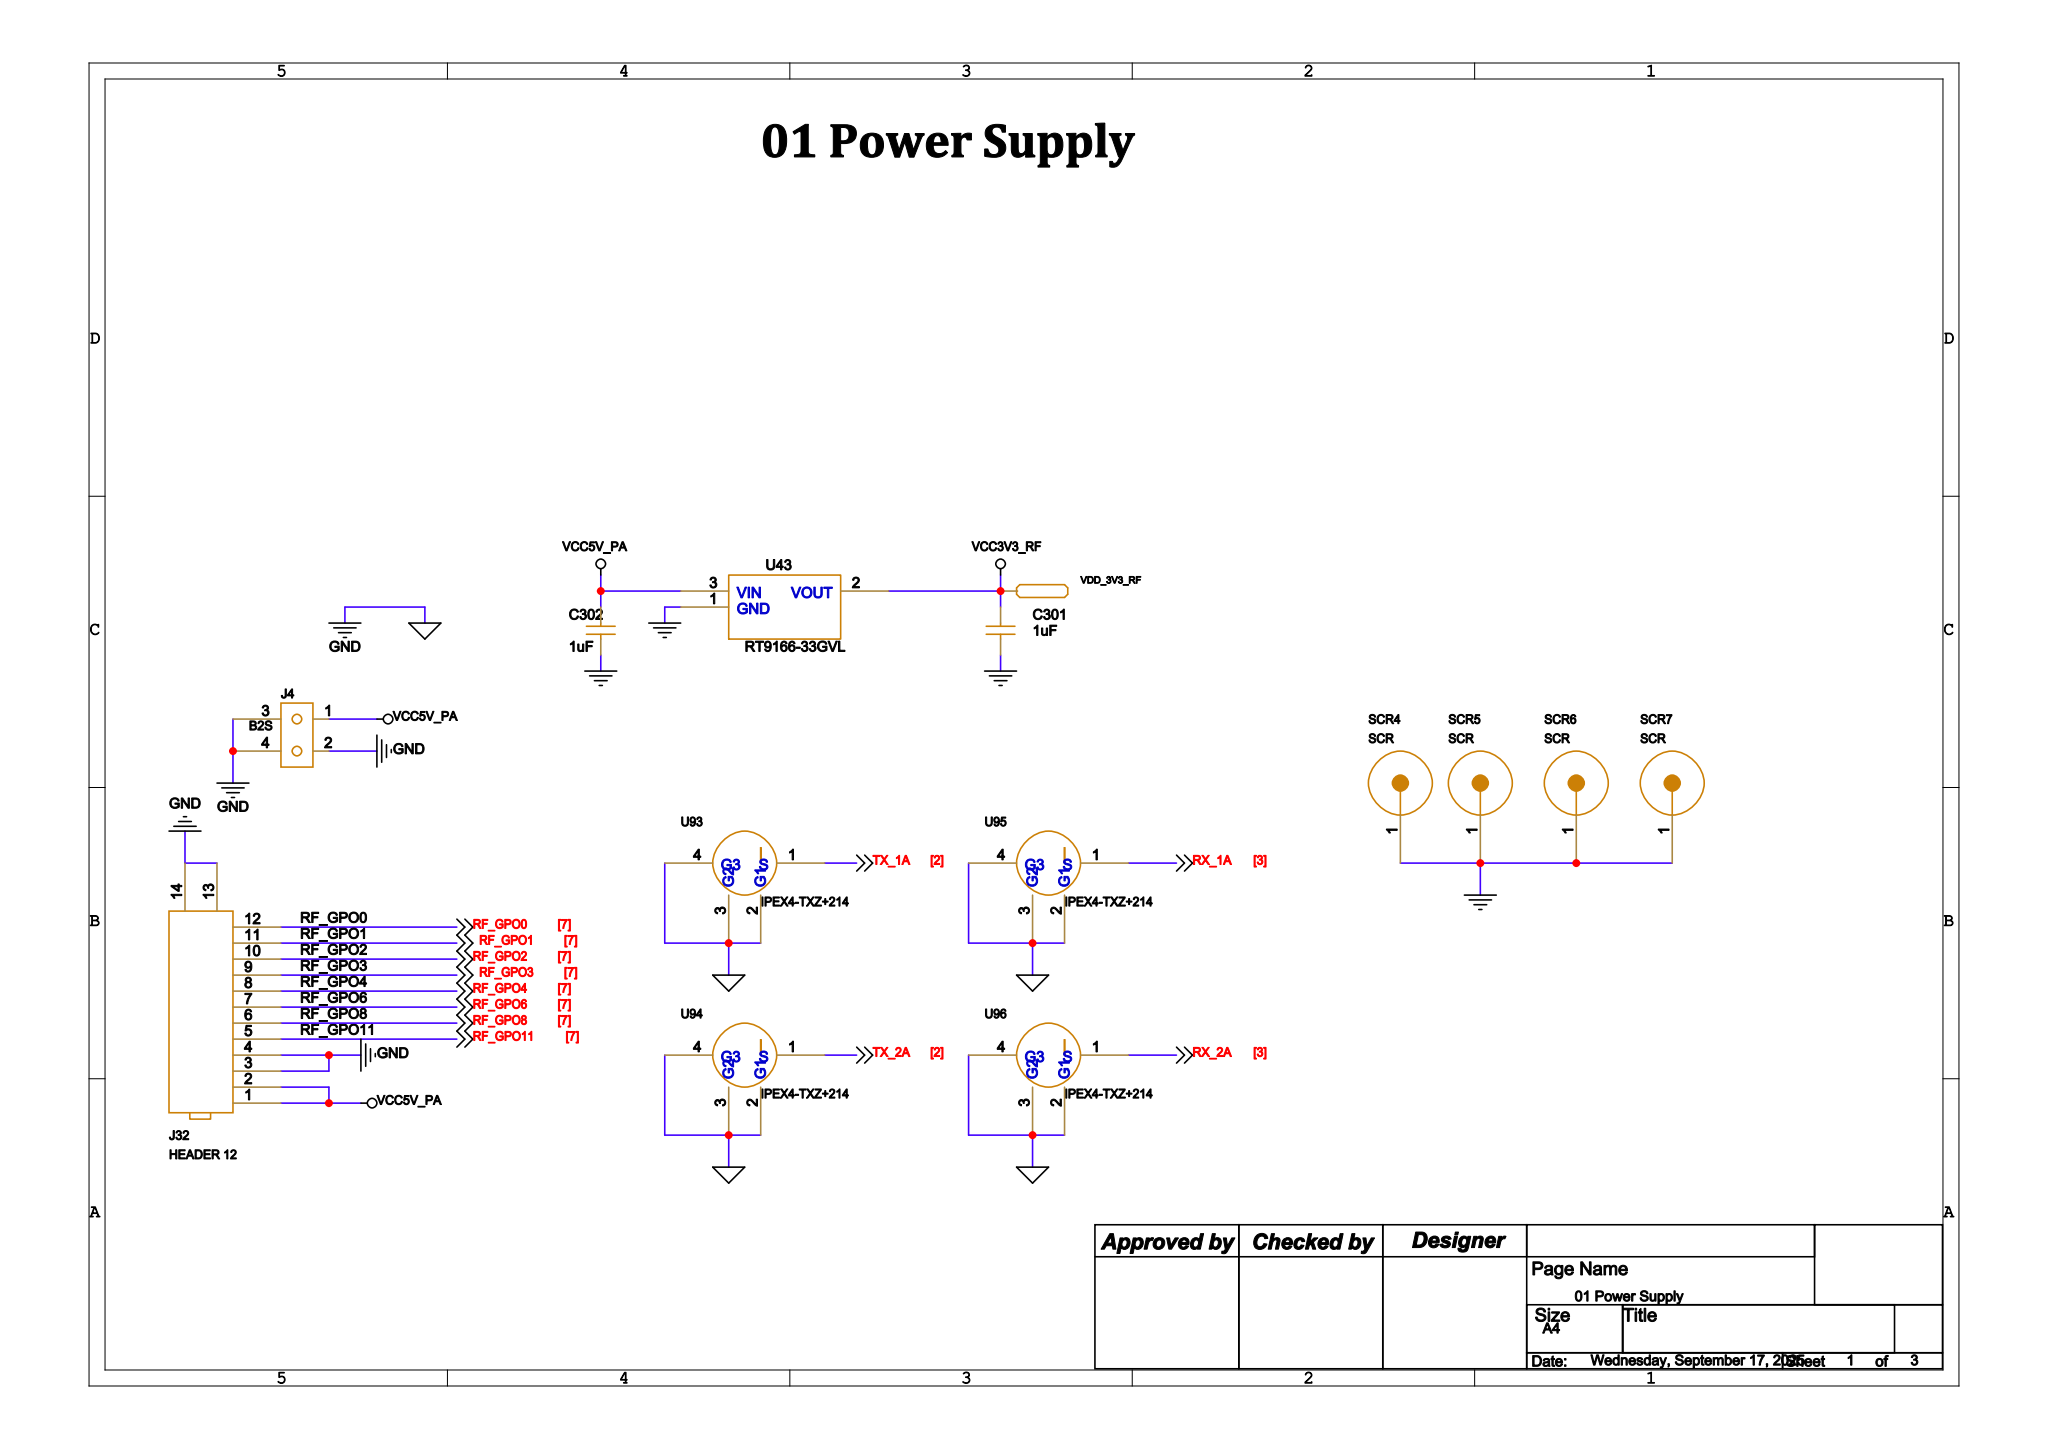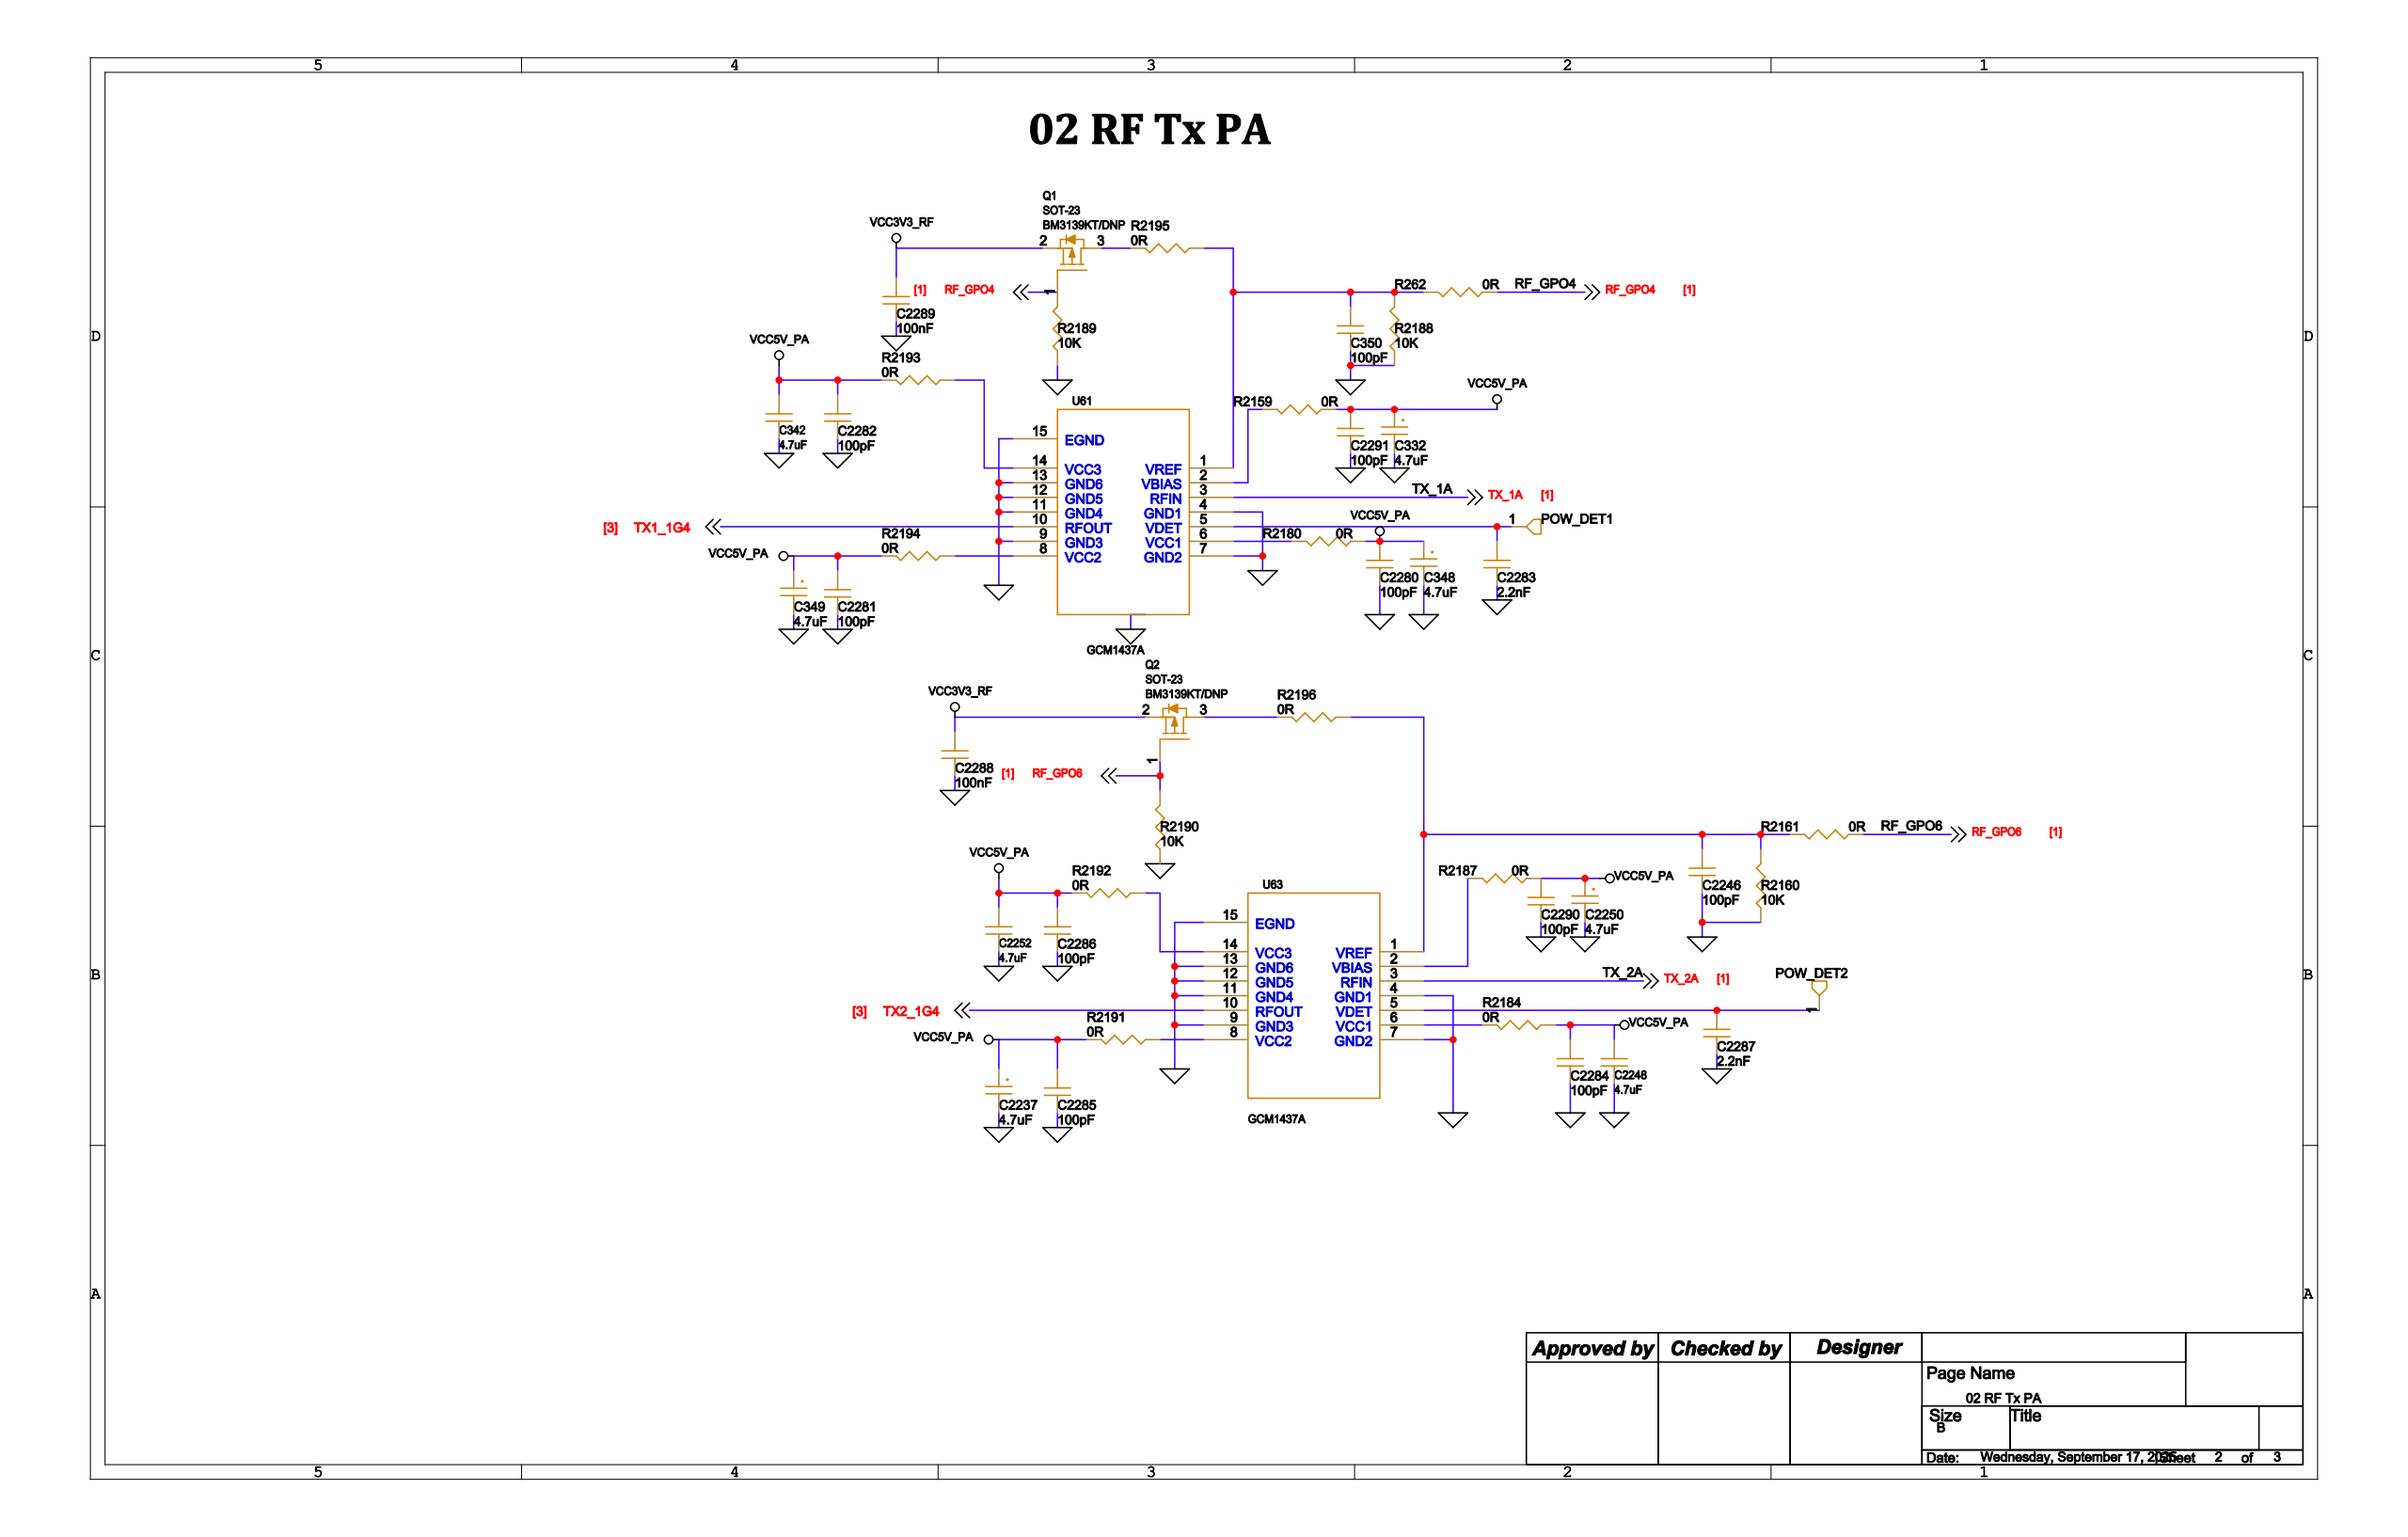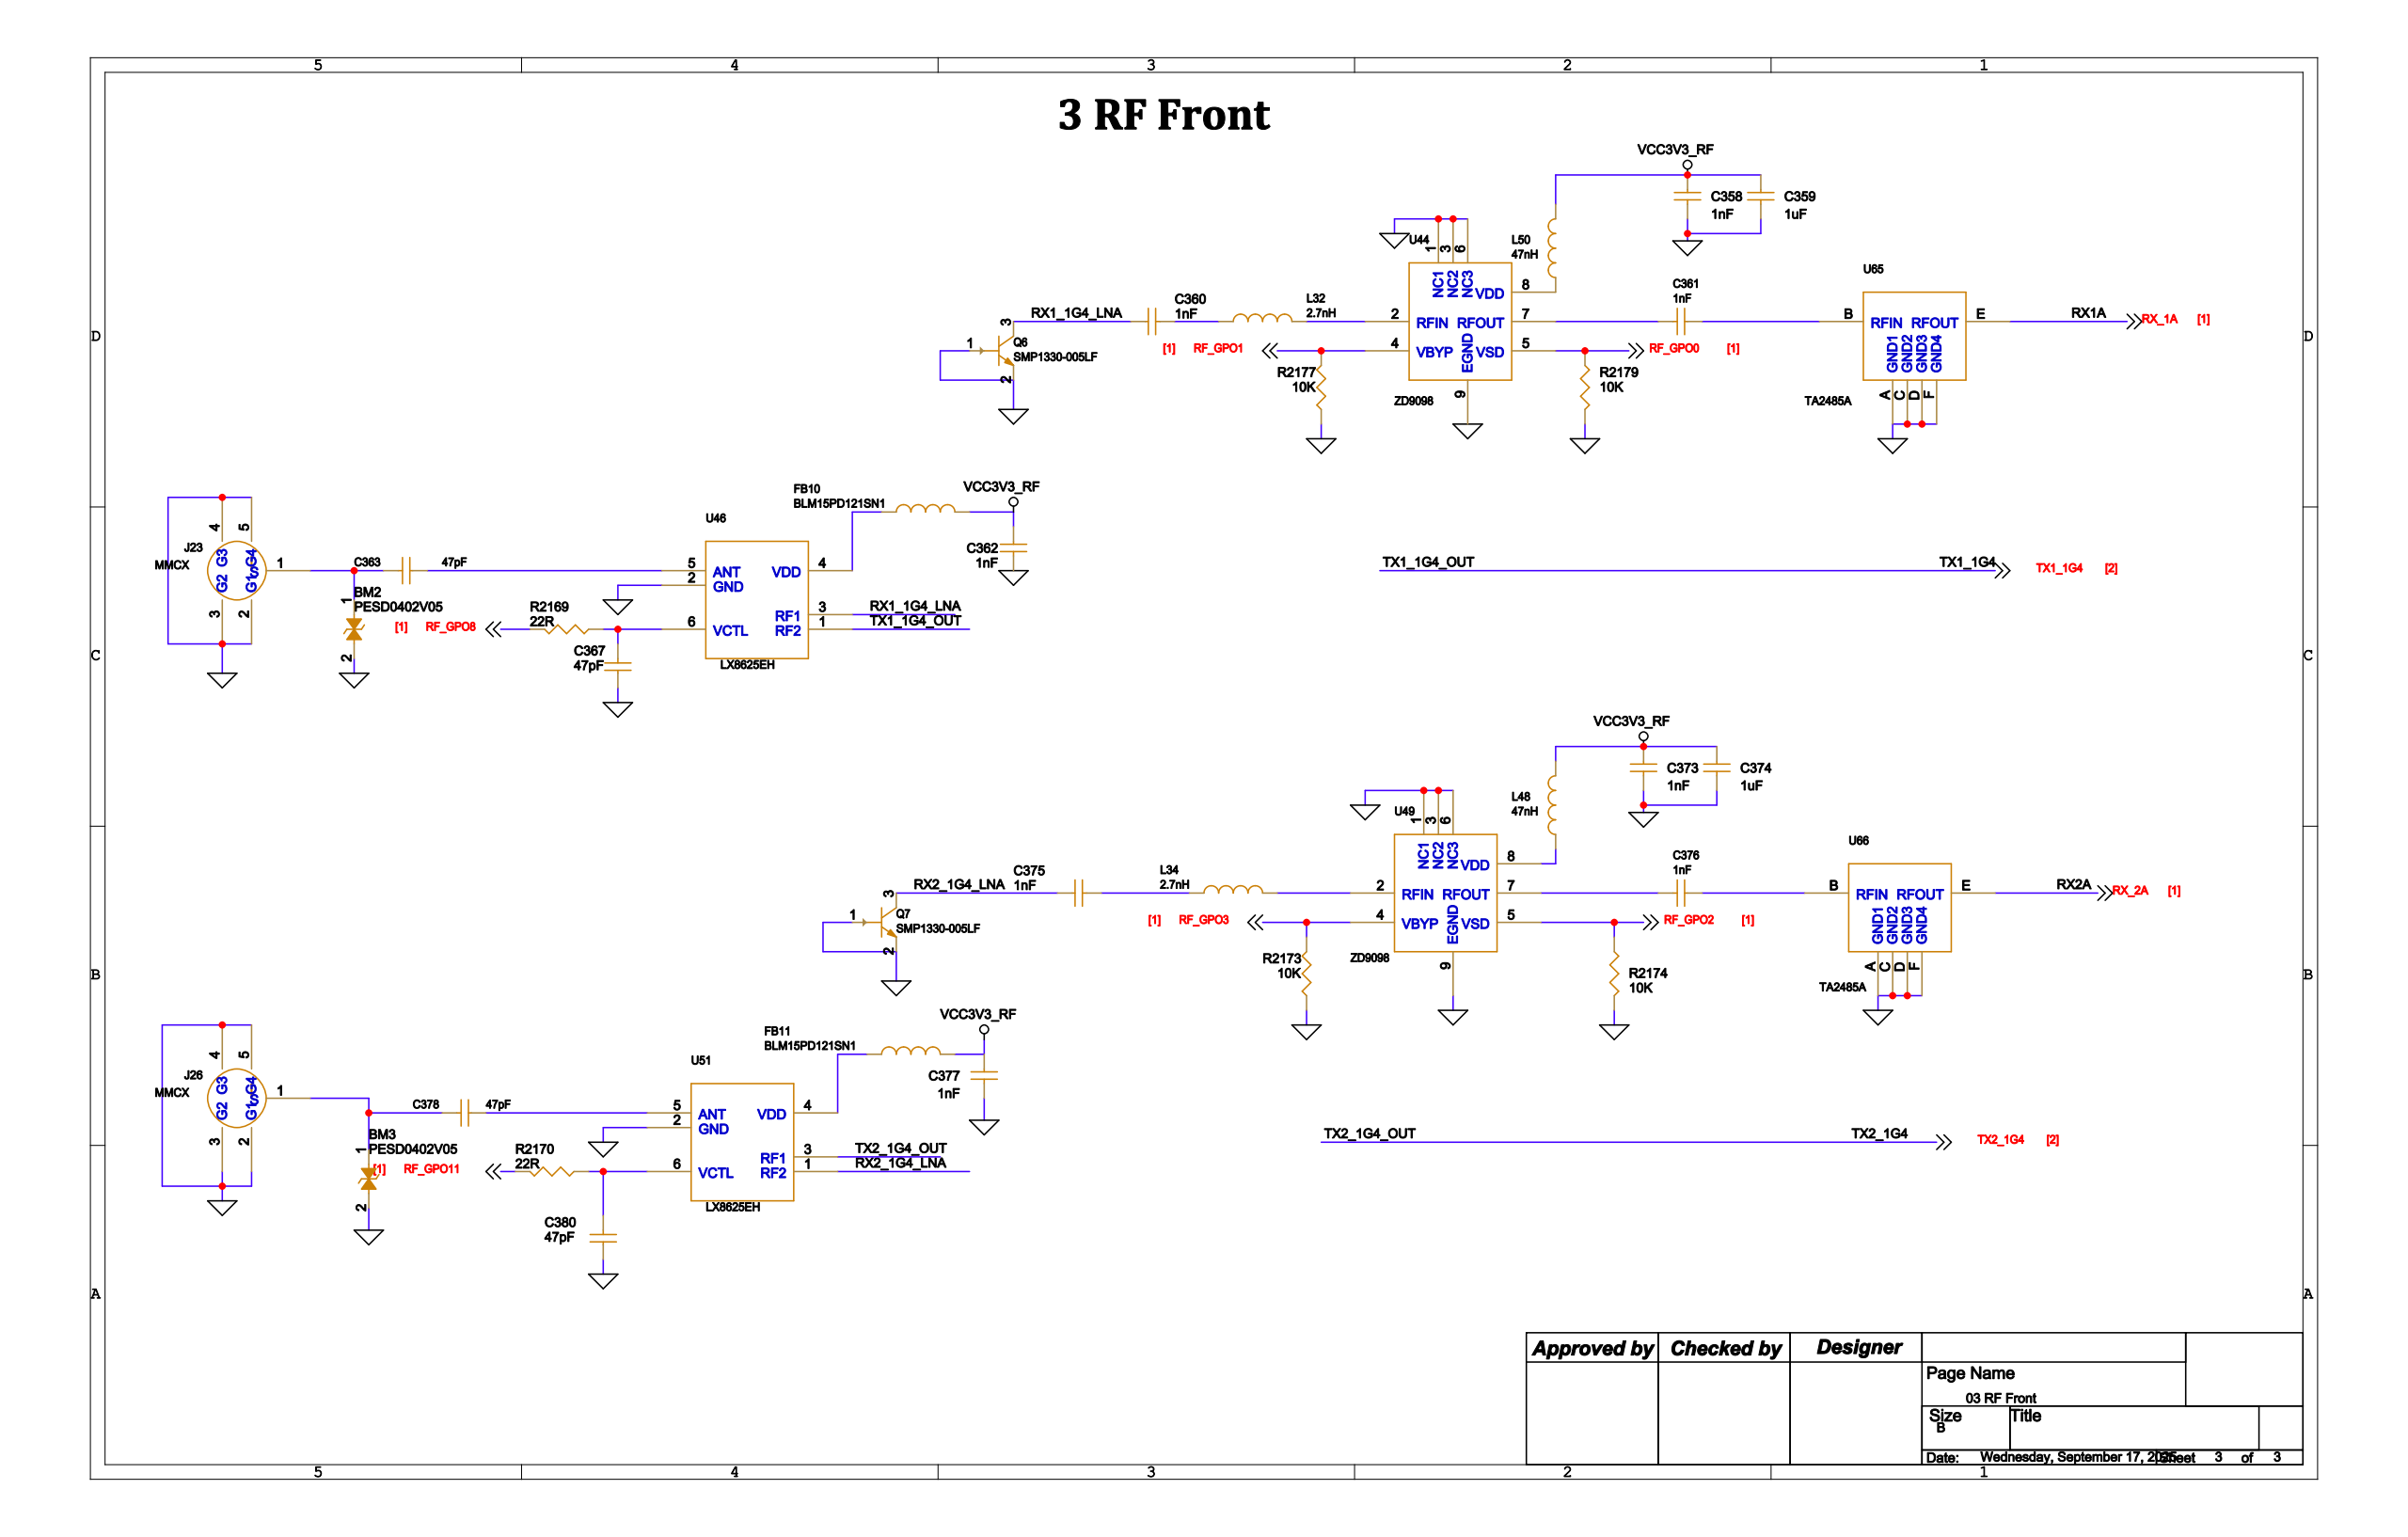Circuit board | Cadence Allegro | 96 parts | 51 nets
Bill of materials:
SYM_NAME,COMP_DEVICE_TYPE,COMP_VALUE,COMP_TOL,COMP_CLASS,REFDES
TVS0402,DIODE ZENER1_4_TVS0402_PESD0402,PESD0402V05,,IC,BM2
TVS0402,DIODE ZENER1_4_TVS0402_PESD0402,PESD0402V05,,IC,BM3
C0402_D,C0603_10NF_C0402_D_1UF,1uF,,IC,C301
C0402_D,C0603_10NF_C0402_D_1UF,1uF,,IC,C302
C0402_D,C0603_0_C0402_D_4.7UF,4.7uF,,IC,C332
C0402_D,CAPACITOR NON-POL_C0402_D_4.7UF,4.7uF,,IC,C342
C0402_D,C0603_0_C0402_D_4.7UF,4.7uF,,IC,C348
C0402_D,C0603_0_C0402_D_4.7UF,4.7uF,,IC,C349
C0402_D,CAP NP_C0402_D_100PF,100pF,,IC,C350
C0402_D,CAPACITOR NON-POL_C0402_D_1NF,1nF,,IC,C358
C0402_D,CAPACITOR NON-POL_C0402_D_1UF,1uF,,IC,C359
C0402_D,CAPACITOR NON-POL_C0402_D_1NF,1nF,,IC,C360
C0402_D,CAPACITOR NON-POL_C0402_D_1NF,1nF,,IC,C361
C0402_D,CAPACITOR NON-POL_C0402_D_1NF,1nF,,IC,C362
C0402_D,CAPACITOR NON-POL_C0402_D_47PF,47pF,,IC,C363
C0402_D,CAPACITOR NON-POL_C0402_D_47PF,47pF,,IC,C367
C0402_D,CAPACITOR NON-POL_C0402_D_1NF,1nF,,IC,C373
C0402_D,CAPACITOR NON-POL_C0402_D_1UF,1uF,,IC,C374
C0402_D,CAPACITOR NON-POL_C0402_D_1NF,1nF,,IC,C375
C0402_D,CAPACITOR NON-POL_C0402_D_1NF,1nF,,IC,C376
C0402_D,CAPACITOR NON-POL_C0402_D_1NF,1nF,,IC,C377
C0402_D,CAPACITOR NON-POL_C0402_D_47PF,47pF,,IC,C378
C0402_D,CAPACITOR NON-POL_C0402_D_47PF,47pF,,IC,C380
C0402_D,C0603_0_C0402_D_4.7UF,4.7uF,,IC,C2237
C0402_D,CAP NP_C0402_D_100PF,100pF,,IC,C2246
C0402_D,CAPACITOR NON-POL_C0402_D_4.7UF,4.7uF,,IC,C2248
C0402_D,C0603_0_C0402_D_4.7UF,4.7uF,,IC,C2250
C0402_D,CAPACITOR NON-POL_C0402_D_4.7UF,4.7uF,,IC,C2252
C0402_D,CAP NP_C0402_D_100PF,100pF,,IC,C2280
C0402_D,CAP NP_C0402_D_100PF,100pF,,IC,C2281
C0402_D,CAP NP_C0402_D_100PF,100pF,,IC,C2282
C0402_D,CAP NP_C0402_D_2.2NF,2.2nF,,IC,C2283
C0402_D,CAP NP_C0402_D_100PF,100pF,,IC,C2284
C0402_D,CAP NP_C0402_D_100PF,100pF,,IC,C2285
C0402_D,CAP NP_C0402_D_100PF,100pF,,IC,C2286
C0402_D,CAP NP_C0402_D_2.2NF,2.2nF,,IC,C2287
C0402_D,CAP NP_C0402_D_100NF,100nF,,IC,C2288
C0402_D,CAP NP_C0402_D_100NF,100nF,,IC,C2289
C0402_D,CAP NP_C0402_D_100PF,100pF,,IC,C2290
C0402_D,CAP NP_C0402_D_100PF,100pF,,IC,C2291
L0402_D,FB0603_1_L0402_D_BLM15PD121SN1_,BLM15PD121SN1,,IC,FB10
L0402_D,FB0603_1_L0402_D_BLM15PD121SN1_,BLM15PD121SN1,,IC,FB11
CNTR-2-1_25-A1251WRS,B2S_0_CNTR-2-1_25-A1251WRS_B2S,B2S,,IC,J4
MMCX008-H,SMA_0_MMCX008-H_MMCX,MMCX,,IC,J23
MMCX008-H,SMA_0_MMCX008-H_MMCX,MMCX,,IC,J26
FPC_0_5_12PIN,HEADER 10X2_5_FPC_0_5_12PIN_HEA,HEADER 12,,IC,J32
L0402_D,INDUCTOR_L0402_D_2.7NH,2.7nH,,IC,L32
L0402_D,INDUCTOR_L0402_D_2.7NH,2.7nH,,IC,L34
L0402_D,INDUCTOR_L0402_D_47NH,47nH,,IC,L48
L0402_D,INDUCTOR_L0402_D_47NH,47nH,,IC,L50
STP40,T POINT F_0_STP40_T POINT F,T POINT F,,IC,POW_DET1
STP40,T POINT F_0_STP40_T POINT F,T POINT F,,IC,POW_DET2
SOT-23,MOSFET P_SOT-23_BM3139KT/DNP,BM3139KT/DNP,,IC,Q1
SOT-23,MOSFET P_SOT-23_BM3139KT/DNP,BM3139KT/DNP,,IC,Q2
SOT-23,TRANSISTOR NPN BC847B 45V SOT23,SMP1330-005LF,,IC,Q6
SOT-23,TRANSISTOR NPN BC847B 45V SOT23,SMP1330-005LF,,IC,Q7
R0402_D,RESISTOR_R0402_D_0R,0R,,IC,R262
R0402_D,RESISTOR_R0402_D_0R,0R,,IC,R2159
R0402_D,RESISTOR_R0402_D_10K,10K,,IC,R2160
R0402_D,RESISTOR_R0402_D_0R,0R,,IC,R2161
R0402_D,RESISTOR_R0402_D_22R,22R,,DISCRETE,R2169
R0402_D,RESISTOR_R0402_D_22R,22R,,DISCRETE,R2170
R0402_D,RESISTOR_R0402_D_10K,10K,,IC,R2173
R0402_D,RESISTOR_R0402_D_10K,10K,,IC,R2174
R0402_D,RESISTOR_R0402_D_10K,10K,,IC,R2177
R0402_D,RESISTOR_R0402_D_10K,10K,,IC,R2179
R0402_D,RESISTOR_R0402_D_0R,0R,,IC,R2180
R0402_D,RESISTOR_R0402_D_0R,0R,,IC,R2184
R0402_D,RESISTOR_R0402_D_0R,0R,,IC,R2187
R0402_D,RESISTOR_R0402_D_10K,10K,,IC,R2188
R0402_D,RESISTOR_R0402_D_10K,10K,,IC,R2189
R0402_D,RESISTOR_R0402_D_10K,10K,,IC,R2190
R0402_D,RESISTOR_R0402_D_0R,0R,,IC,R2191
R0402_D,RESISTOR_R0402_D_0R,0R,,IC,R2192
R0402_D,RESISTOR_R0402_D_0R,0R,,IC,R2193
R0402_D,RESISTOR_R0402_D_0R,0R,,IC,R2194
R0402_D,RESISTOR_R0402_D_0R,0R,,IC,R2195
R0402_D,RESISTOR_R0402_D_0R,0R,,IC,R2196
HOLE2_2_4,CC_HOLE2_2_4_SCR,SCR,,IC,SCR4
HOLE2_2_4,CC_HOLE2_2_4_SCR,SCR,,IC,SCR5
HOLE2_2_4,CC_HOLE2_2_4_SCR,SCR,,IC,SCR6
HOLE2_2_4,CC_HOLE2_2_4_SCR,SCR,,IC,SCR7
SOT-23,XC6206_SOT-23_RT9166-33GVL,RT9166-33GVL,,IC,U43
DFN2X2-8P,ZD9098_DFN2X2-8P_ZD9098,ZD9098,,IC,U44
DFN6_1_1_0_7MM,FM8625H_DFN6_1_1_0_7MM_LX8625EH,LX8625EH,,IC,U46
DFN2X2-8P,ZD9098_DFN2X2-8P_ZD9098,ZD9098,,IC,U49
DFN6_1_1_0_7MM,FM8625H_DFN6_1_1_0_7MM_LX8625EH,LX8625EH,,IC,U51
PA-14-1_06-GCM1437A,GWM1529_0_PA-14-1_06-GCM1437A_G,GCM1437A,,IC,U61
PA-14-1_06-GCM1437A,GWM1529_0_PA-14-1_06-GCM1437A_G,GCM1437A,,IC,U63
TA2494A,DAC121S_0_TA2494A_TA2485A,TA2485A,,IC,U65
TA2494A,DAC121S_0_TA2494A_TA2485A,TA2485A,,IC,U66
IPEX4-2,IPEX_0_IPEX4-2_IPEX4-TXZ+214,IPEX4-TXZ+214,,IC,U93
IPEX4-2,IPEX_2_IPEX4-2_IPEX4-TXZ+214,IPEX4-TXZ+214,,IC,U94
IPEX4-2,IPEX_1_IPEX4-2_IPEX4-TXZ+214,IPEX4-TXZ+214,,IC,U95
IPEX4-2,IPEX_3_IPEX4-2_IPEX4-TXZ+214,IPEX4-TXZ+214,,IC,U96
LTPT28C49P,LABTESTPOINT_LTPT28C49P_LABTEST,LABTESTPOINT,,IC,VDD_3V3_RF
Netlist (net: part-pin ...):
VCC5V_PA: C302-1 C332-1 C342-2 C348-1 C349-1 C2237-1 C2248-2 C2250-1 C2252-2 C2280-2 C2281-2 C2282-2 C2284-2 C2285-2 C2286-2 C2290-2 C2291-2 J4-1 J32-1 J32-2 R2159-2 R2180-2 R2184-2 R2187-2 R2191-1 R2192-1 R2193-1 R2194-1 U43-3
GND: BM2-2 BM3-2 C301-2 C302-2 C332-2 C342-1 C348-2 C349-2 C350-1 C358-2 C359-2 C362-2 C367-1 C373-2 C374-2 C377-2 C380-1 C2237-2 C2246-1 C2248-1 C2250-2 C2252-1 C2280-1 C2281-1 C2282-1 C2283-1 C2284-1 C2285-1 C2286-1 C2287-1 C2288-1 C2289-1 C2290-1 C2291-1 J4-2 J4-3 J4-4 J23-2 J23-3 J23-4 J23-5 J26-2 J26-3 J26-4 J26-5 J32-3 J32-4 J32-13 J32-14 Q6-1 Q6-2 Q7-1 Q7-2 R2160-2 R2173-1 R2174-2 R2177-1 R2179-2 R2188-2 R2189-2 R2190-2 SCR4-1 SCR5-1 SCR6-1 SCR7-1 U43-1 U44-1 U44-3 U44-6 U44-9 U46-2 U49-1 U49-3 U49-6 U49-9 U51-2 U61-4 U61-7 U61-9 U61-11 U61-12 U61-13 U61-15 U63-4 U63-7 U63-9 U63-11 U63-12 U63-13 U63-15 U65-A U65-C U65-D U65-F U66-A U66-C U66-D U66-F U93-2 U93-3 U93-4 U94-2 U94-3 U94-4 U95-2 U95-3 U95-4 U96-2 U96-3 U96-4
TX_1A: U61-3 U93-1
TX_2A: U63-3 U94-1
RX_1A: U65-E U95-1
RX_2A: U66-E U96-1
N49088438: BM2-1 C363-2 J23-1
N38199412: BM3-1 C378-2 J26-1
RX1_1G4_LNA: C360-1 Q6-3 U46-3
RX2_1G4_LNA: C375-1 Q7-3 U51-1
VCC3V3_RF: C301-1 C358-1 C359-1 C362-1 C373-1 C374-1 C377-1 C2288-2 C2289-2 FB10-2 FB11-2 L48-2 L50-2 Q1-2 Q2-2 U43-2 VDD_3V3_RF-1
N50320358: Q1-3 R2195-1
RF_GPO4: J32-8 Q1-1 R262-2 R2189-1
N50320597: Q2-3 R2196-1
RF_GPO6: J32-7 Q2-1 R2161-2 R2190-1
N50309666: C2283-2 POW_DET1-1 U61-5
N50288038: C2287-2 POW_DET2-1 U63-5
TX1_1G4: U46-1 U61-10
N50313370: R2159-1 U61-2
N50050224: R2180-1 U61-6
N50323845: R2194-2 U61-8
N50056105: R2193-2 U61-14
N49200262: C350-2 R262-1 R2188-1 R2195-2 U61-1
TX2_1G4: U51-3 U63-10
N50317954: R2187-1 U63-2
N50316607: R2184-1 U63-6
N50323373: R2191-2 U63-8
N50316807: R2192-2 U63-14
N50288008: C2246-2 R2160-1 R2161-1 R2196-2 U63-1
RF_GPO2: J32-10 R2174-1 U49-5
RF_GPO1: J32-11 R2177-2 U44-4
RF_GPO0: J32-12 R2179-1 U44-5
RF_GPO11: J32-5 R2170-2
RF_GPO8: J32-6 R2169-1
RF_GPO3: J32-9 R2173-2 U49-4
N38188746: C363-1 U46-5
N50020375: C367-2 R2169-2 U46-6
N49090908: FB10-1 U46-4
N50289371: C378-1 U51-5
N50289399: C380-2 R2170-1 U51-6
N50289343: FB11-1 U51-4
N50025513: C361-1 U65-B
N50058764: C376-1 U66-B
N49193940: C360-2 L32-1
N49181397: L32-2 U44-2
N50289007: C375-2 L34-1
N49181793: L34-2 U49-2
N50084496: L48-1 U49-8
N501130470: L50-1 U44-8
N50025516: C361-2 U44-7
N49181807: C376-2 U49-7